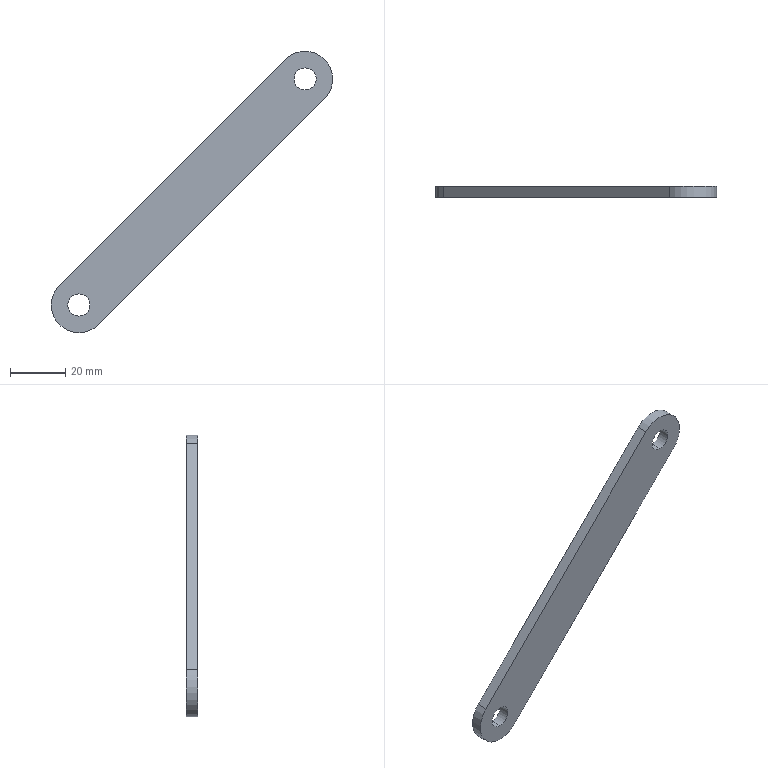Part | SolidWorks | features Extrusion 1 | 1 solid | 11 faces | box 101.635 x 4 x 101.635 mm | volume 10090 mm3 | cylinder 7 | plane 4 | commonest cylinder face diameters 8 x4 20 x3
STEP:
#1=CARTESIAN_POINT('',(-36.47,4.,-44.817));
#2=VERTEX_POINT('',#1);
#3=CARTESIAN_POINT('',(-36.47,4.,-36.817));
#4=VERTEX_POINT('',#3);
#5=CARTESIAN_POINT('',(-36.47,4.,-40.817));
#6=DIRECTION('',(0.,1.,0.));
#7=DIRECTION('',(0.,0.,1.));
#8=AXIS2_PLACEMENT_3D('',#5,#6,#7);
#9=CIRCLE('',#8,4.);
#10=EDGE_CURVE('',#2,#4,#9,.T.);
#11=ORIENTED_EDGE('',*,*,#10,.T.);
#12=CARTESIAN_POINT('',(-36.47,0.,-36.817));
#13=VERTEX_POINT('',#12);
#14=CARTESIAN_POINT('',(-36.47,4.,-36.817));
#15=DIRECTION('',(0.,-1.,0.));
#16=VECTOR('',#15,1000.);
#17=LINE('',#14,#16);
#18=EDGE_CURVE('',#4,#13,#17,.T.);
#19=ORIENTED_EDGE('',*,*,#18,.T.);
#20=CARTESIAN_POINT('',(-36.47,0.,-44.817));
#21=VERTEX_POINT('',#20);
#22=CARTESIAN_POINT('',(-36.47,0.,-40.817));
#23=DIRECTION('',(0.,1.,0.));
#24=DIRECTION('',(0.,0.,1.));
#25=AXIS2_PLACEMENT_3D('',#22,#23,#24);
#26=CIRCLE('',#25,4.);
#27=EDGE_CURVE('',#21,#13,#26,.T.);
#28=ORIENTED_EDGE('',*,*,#27,.F.);
#29=CARTESIAN_POINT('',(-36.47,4.,-44.817));
#30=DIRECTION('',(0.,-1.,0.));
#31=VECTOR('',#30,1000.);
#32=LINE('',#29,#31);
#33=EDGE_CURVE('',#2,#21,#32,.T.);
#34=ORIENTED_EDGE('',*,*,#33,.F.);
#35=EDGE_LOOP('',(#11,#19,#28,#34));
#36=FACE_OUTER_BOUND('',#35,.T.);
#37=CARTESIAN_POINT('',(-36.47,4.,-40.817));
#38=DIRECTION('',(0.,-1.,0.));
#39=DIRECTION('',(0.,0.,-1.));
#40=AXIS2_PLACEMENT_3D('',#37,#38,#39);
#41=CYLINDRICAL_SURFACE('',#40,4.);
#42=ADVANCED_FACE('',(#36),#41,.F.);
#43=CARTESIAN_POINT('',(45.165,4.,36.817));
#44=VERTEX_POINT('',#43);
#45=CARTESIAN_POINT('',(45.165,4.,44.817));
#46=VERTEX_POINT('',#45);
#47=CARTESIAN_POINT('',(45.165,4.,40.817));
#48=DIRECTION('',(0.,1.,0.));
#49=DIRECTION('',(0.,0.,1.));
#50=AXIS2_PLACEMENT_3D('',#47,#48,#49);
#51=CIRCLE('',#50,4.);
#52=EDGE_CURVE('',#44,#46,#51,.T.);
#53=ORIENTED_EDGE('',*,*,#52,.T.);
#54=CARTESIAN_POINT('',(45.165,0.,44.817));
#55=VERTEX_POINT('',#54);
#56=CARTESIAN_POINT('',(45.165,4.,44.817));
#57=DIRECTION('',(0.,-1.,0.));
#58=VECTOR('',#57,1000.);
#59=LINE('',#56,#58);
#60=EDGE_CURVE('',#46,#55,#59,.T.);
#61=ORIENTED_EDGE('',*,*,#60,.T.);
#62=CARTESIAN_POINT('',(45.165,0.,36.817));
#63=VERTEX_POINT('',#62);
#64=CARTESIAN_POINT('',(45.165,0.,40.817));
#65=DIRECTION('',(0.,1.,0.));
#66=DIRECTION('',(0.,0.,1.));
#67=AXIS2_PLACEMENT_3D('',#64,#65,#66);
#68=CIRCLE('',#67,4.);
#69=EDGE_CURVE('',#63,#55,#68,.T.);
#70=ORIENTED_EDGE('',*,*,#69,.F.);
#71=CARTESIAN_POINT('',(45.165,4.,36.817));
#72=DIRECTION('',(0.,-1.,0.));
#73=VECTOR('',#72,1000.);
#74=LINE('',#71,#73);
#75=EDGE_CURVE('',#44,#63,#74,.T.);
#76=ORIENTED_EDGE('',*,*,#75,.F.);
#77=EDGE_LOOP('',(#53,#61,#70,#76));
#78=FACE_OUTER_BOUND('',#77,.T.);
#79=CARTESIAN_POINT('',(45.165,4.,40.817));
#80=DIRECTION('',(0.,-1.,0.));
#81=DIRECTION('',(0.,0.,-1.));
#82=AXIS2_PLACEMENT_3D('',#79,#80,#81);
#83=CYLINDRICAL_SURFACE('',#82,4.);
#84=ADVANCED_FACE('',(#78),#83,.F.);
#85=CARTESIAN_POINT('',(-36.47,4.,-50.817));
#86=VERTEX_POINT('',#85);
#87=CARTESIAN_POINT('',(-43.541,4.,-33.746));
#88=VERTEX_POINT('',#87);
#89=CARTESIAN_POINT('',(-36.47,4.,-40.817));
#90=DIRECTION('',(0.,1.,0.));
#91=DIRECTION('',(0.,0.,1.));
#92=AXIS2_PLACEMENT_3D('',#89,#90,#91);
#93=CIRCLE('',#92,10.);
#94=EDGE_CURVE('',#86,#88,#93,.T.);
#95=ORIENTED_EDGE('',*,*,#94,.F.);
#96=CARTESIAN_POINT('',(-36.47,0.,-50.817));
#97=VERTEX_POINT('',#96);
#98=CARTESIAN_POINT('',(-36.47,4.,-50.817));
#99=DIRECTION('',(0.,-1.,0.));
#100=VECTOR('',#99,1000.);
#101=LINE('',#98,#100);
#102=EDGE_CURVE('',#86,#97,#101,.T.);
#103=ORIENTED_EDGE('',*,*,#102,.T.);
#104=CARTESIAN_POINT('',(-43.541,0.,-33.746));
#105=VERTEX_POINT('',#104);
#106=CARTESIAN_POINT('',(-36.47,0.,-40.817));
#107=DIRECTION('',(0.,1.,0.));
#108=DIRECTION('',(0.,0.,1.));
#109=AXIS2_PLACEMENT_3D('',#106,#107,#108);
#110=CIRCLE('',#109,10.);
#111=EDGE_CURVE('',#97,#105,#110,.T.);
#112=ORIENTED_EDGE('',*,*,#111,.T.);
#113=CARTESIAN_POINT('',(-43.541,4.,-33.746));
#114=DIRECTION('',(0.,-1.,0.));
#115=VECTOR('',#114,1000.);
#116=LINE('',#113,#115);
#117=EDGE_CURVE('',#88,#105,#116,.T.);
#118=ORIENTED_EDGE('',*,*,#117,.F.);
#119=EDGE_LOOP('',(#95,#103,#112,#118));
#120=FACE_OUTER_BOUND('',#119,.T.);
#121=CARTESIAN_POINT('',(-36.47,4.,-40.817));
#122=DIRECTION('',(0.,-1.,0.));
#123=DIRECTION('',(0.,0.,-1.));
#124=AXIS2_PLACEMENT_3D('',#121,#122,#123);
#125=CYLINDRICAL_SURFACE('',#124,10.);
#126=ADVANCED_FACE('',(#120),#125,.T.);
#127=ORIENTED_EDGE('',*,*,#52,.F.);
#128=CARTESIAN_POINT('',(45.165,4.,40.817));
#129=DIRECTION('',(0.,1.,0.));
#130=DIRECTION('',(0.,0.,1.));
#131=AXIS2_PLACEMENT_3D('',#128,#129,#130);
#132=CIRCLE('',#131,4.);
#133=EDGE_CURVE('',#46,#44,#132,.T.);
#134=ORIENTED_EDGE('',*,*,#133,.F.);
#135=EDGE_LOOP('',(#127,#134));
#136=FACE_BOUND('',#135,.T.);
#137=CARTESIAN_POINT('',(38.094,4.,47.889));
#138=VERTEX_POINT('',#137);
#139=CARTESIAN_POINT('',(52.236,4.,33.746));
#140=VERTEX_POINT('',#139);
#141=CARTESIAN_POINT('',(45.165,4.,40.817));
#142=DIRECTION('',(0.,1.,0.));
#143=DIRECTION('',(0.,0.,1.));
#144=AXIS2_PLACEMENT_3D('',#141,#142,#143);
#145=CIRCLE('',#144,10.);
#146=EDGE_CURVE('',#138,#140,#145,.T.);
#147=ORIENTED_EDGE('',*,*,#146,.T.);
#148=CARTESIAN_POINT('',(-29.399,4.,-47.889));
#149=VERTEX_POINT('',#148);
#150=CARTESIAN_POINT('',(52.236,4.,33.746));
#151=DIRECTION('',(-0.7071,0.,-0.7071));
#152=VECTOR('',#151,1000.);
#153=LINE('',#150,#152);
#154=EDGE_CURVE('',#140,#149,#153,.T.);
#155=ORIENTED_EDGE('',*,*,#154,.T.);
#156=CARTESIAN_POINT('',(-36.47,4.,-40.817));
#157=DIRECTION('',(0.,1.,0.));
#158=DIRECTION('',(0.,0.,1.));
#159=AXIS2_PLACEMENT_3D('',#156,#157,#158);
#160=CIRCLE('',#159,10.);
#161=EDGE_CURVE('',#149,#86,#160,.T.);
#162=ORIENTED_EDGE('',*,*,#161,.T.);
#163=ORIENTED_EDGE('',*,*,#94,.T.);
#164=CARTESIAN_POINT('',(38.094,4.,47.889));
#165=DIRECTION('',(0.7071,0.,0.7071));
#166=VECTOR('',#165,1000.);
#167=LINE('',#164,#166);
#168=EDGE_CURVE('',#88,#138,#167,.T.);
#169=ORIENTED_EDGE('',*,*,#168,.T.);
#170=EDGE_LOOP('',(#147,#155,#162,#163,#169));
#171=FACE_OUTER_BOUND('',#170,.T.);
#172=ORIENTED_EDGE('',*,*,#10,.F.);
#173=CARTESIAN_POINT('',(-36.47,4.,-40.817));
#174=DIRECTION('',(0.,1.,0.));
#175=DIRECTION('',(0.,0.,1.));
#176=AXIS2_PLACEMENT_3D('',#173,#174,#175);
#177=CIRCLE('',#176,4.);
#178=EDGE_CURVE('',#4,#2,#177,.T.);
#179=ORIENTED_EDGE('',*,*,#178,.F.);
#180=EDGE_LOOP('',(#172,#179));
#181=FACE_BOUND('',#180,.T.);
#182=CARTESIAN_POINT('',(45.165,4.,40.817));
#183=DIRECTION('',(0.,1.,0.));
#184=DIRECTION('',(0.,0.,1.));
#185=AXIS2_PLACEMENT_3D('',#182,#183,#184);
#186=PLANE('',#185);
#187=ADVANCED_FACE('',(#136,#171,#181),#186,.T.);
#188=CARTESIAN_POINT('',(38.094,0.,47.889));
#189=VERTEX_POINT('',#188);
#190=CARTESIAN_POINT('',(52.236,0.,33.746));
#191=VERTEX_POINT('',#190);
#192=CARTESIAN_POINT('',(45.165,0.,40.817));
#193=DIRECTION('',(0.,1.,0.));
#194=DIRECTION('',(0.,0.,1.));
#195=AXIS2_PLACEMENT_3D('',#192,#193,#194);
#196=CIRCLE('',#195,10.);
#197=EDGE_CURVE('',#189,#191,#196,.T.);
#198=ORIENTED_EDGE('',*,*,#197,.F.);
#199=CARTESIAN_POINT('',(38.094,0.,47.889));
#200=DIRECTION('',(0.7071,0.,0.7071));
#201=VECTOR('',#200,1000.);
#202=LINE('',#199,#201);
#203=EDGE_CURVE('',#105,#189,#202,.T.);
#204=ORIENTED_EDGE('',*,*,#203,.F.);
#205=ORIENTED_EDGE('',*,*,#111,.F.);
#206=CARTESIAN_POINT('',(-29.399,0.,-47.889));
#207=VERTEX_POINT('',#206);
#208=CARTESIAN_POINT('',(-36.47,0.,-40.817));
#209=DIRECTION('',(0.,1.,0.));
#210=DIRECTION('',(0.,0.,1.));
#211=AXIS2_PLACEMENT_3D('',#208,#209,#210);
#212=CIRCLE('',#211,10.);
#213=EDGE_CURVE('',#207,#97,#212,.T.);
#214=ORIENTED_EDGE('',*,*,#213,.F.);
#215=CARTESIAN_POINT('',(52.236,0.,33.746));
#216=DIRECTION('',(-0.7071,0.,-0.7071));
#217=VECTOR('',#216,1000.);
#218=LINE('',#215,#217);
#219=EDGE_CURVE('',#191,#207,#218,.T.);
#220=ORIENTED_EDGE('',*,*,#219,.F.);
#221=EDGE_LOOP('',(#198,#204,#205,#214,#220));
#222=FACE_OUTER_BOUND('',#221,.T.);
#223=ORIENTED_EDGE('',*,*,#69,.T.);
#224=CARTESIAN_POINT('',(45.165,0.,40.817));
#225=DIRECTION('',(0.,1.,0.));
#226=DIRECTION('',(0.,0.,1.));
#227=AXIS2_PLACEMENT_3D('',#224,#225,#226);
#228=CIRCLE('',#227,4.);
#229=EDGE_CURVE('',#55,#63,#228,.T.);
#230=ORIENTED_EDGE('',*,*,#229,.T.);
#231=EDGE_LOOP('',(#223,#230));
#232=FACE_BOUND('',#231,.T.);
#233=ORIENTED_EDGE('',*,*,#27,.T.);
#234=CARTESIAN_POINT('',(-36.47,0.,-40.817));
#235=DIRECTION('',(0.,1.,0.));
#236=DIRECTION('',(0.,0.,1.));
#237=AXIS2_PLACEMENT_3D('',#234,#235,#236);
#238=CIRCLE('',#237,4.);
#239=EDGE_CURVE('',#13,#21,#238,.T.);
#240=ORIENTED_EDGE('',*,*,#239,.T.);
#241=EDGE_LOOP('',(#233,#240));
#242=FACE_BOUND('',#241,.T.);
#243=CARTESIAN_POINT('',(45.165,0.,40.817));
#244=DIRECTION('',(0.,1.,0.));
#245=DIRECTION('',(0.,0.,1.));
#246=AXIS2_PLACEMENT_3D('',#243,#244,#245);
#247=PLANE('',#246);
#248=ADVANCED_FACE('',(#222,#232,#242),#247,.F.);
#249=ORIENTED_EDGE('',*,*,#197,.T.);
#250=CARTESIAN_POINT('',(52.236,4.,33.746));
#251=DIRECTION('',(0.,-1.,0.));
#252=VECTOR('',#251,1000.);
#253=LINE('',#250,#252);
#254=EDGE_CURVE('',#140,#191,#253,.T.);
#255=ORIENTED_EDGE('',*,*,#254,.F.);
#256=ORIENTED_EDGE('',*,*,#146,.F.);
#257=CARTESIAN_POINT('',(38.094,4.,47.889));
#258=DIRECTION('',(0.,-1.,0.));
#259=VECTOR('',#258,1000.);
#260=LINE('',#257,#259);
#261=EDGE_CURVE('',#138,#189,#260,.T.);
#262=ORIENTED_EDGE('',*,*,#261,.T.);
#263=EDGE_LOOP('',(#249,#255,#256,#262));
#264=FACE_OUTER_BOUND('',#263,.T.);
#265=CARTESIAN_POINT('',(45.165,4.,40.817));
#266=DIRECTION('',(0.,-1.,0.));
#267=DIRECTION('',(0.,0.,-1.));
#268=AXIS2_PLACEMENT_3D('',#265,#266,#267);
#269=CYLINDRICAL_SURFACE('',#268,10.);
#270=ADVANCED_FACE('',(#264),#269,.T.);
#271=ORIENTED_EDGE('',*,*,#219,.T.);
#272=CARTESIAN_POINT('',(-29.399,4.,-47.889));
#273=DIRECTION('',(0.,-1.,0.));
#274=VECTOR('',#273,1000.);
#275=LINE('',#272,#274);
#276=EDGE_CURVE('',#149,#207,#275,.T.);
#277=ORIENTED_EDGE('',*,*,#276,.F.);
#278=ORIENTED_EDGE('',*,*,#154,.F.);
#279=ORIENTED_EDGE('',*,*,#254,.T.);
#280=EDGE_LOOP('',(#271,#277,#278,#279));
#281=FACE_OUTER_BOUND('',#280,.T.);
#282=CARTESIAN_POINT('',(52.236,4.,33.746));
#283=DIRECTION('',(-0.7071,0.,0.7071));
#284=DIRECTION('',(0.7071,0.,0.7071));
#285=AXIS2_PLACEMENT_3D('',#282,#283,#284);
#286=PLANE('',#285);
#287=ADVANCED_FACE('',(#281),#286,.F.);
#288=ORIENTED_EDGE('',*,*,#102,.F.);
#289=ORIENTED_EDGE('',*,*,#161,.F.);
#290=ORIENTED_EDGE('',*,*,#276,.T.);
#291=ORIENTED_EDGE('',*,*,#213,.T.);
#292=EDGE_LOOP('',(#288,#289,#290,#291));
#293=FACE_OUTER_BOUND('',#292,.T.);
#294=CARTESIAN_POINT('',(-36.47,4.,-40.817));
#295=DIRECTION('',(0.,-1.,0.));
#296=DIRECTION('',(0.,0.,-1.));
#297=AXIS2_PLACEMENT_3D('',#294,#295,#296);
#298=CYLINDRICAL_SURFACE('',#297,10.);
#299=ADVANCED_FACE('',(#293),#298,.T.);
#300=ORIENTED_EDGE('',*,*,#203,.T.);
#301=ORIENTED_EDGE('',*,*,#261,.F.);
#302=ORIENTED_EDGE('',*,*,#168,.F.);
#303=ORIENTED_EDGE('',*,*,#117,.T.);
#304=EDGE_LOOP('',(#300,#301,#302,#303));
#305=FACE_OUTER_BOUND('',#304,.T.);
#306=CARTESIAN_POINT('',(38.094,4.,47.889));
#307=DIRECTION('',(0.7071,0.,-0.7071));
#308=DIRECTION('',(-0.7071,0.,-0.7071));
#309=AXIS2_PLACEMENT_3D('',#306,#307,#308);
#310=PLANE('',#309);
#311=ADVANCED_FACE('',(#305),#310,.F.);
#312=ORIENTED_EDGE('',*,*,#60,.F.);
#313=ORIENTED_EDGE('',*,*,#133,.T.);
#314=ORIENTED_EDGE('',*,*,#75,.T.);
#315=ORIENTED_EDGE('',*,*,#229,.F.);
#316=EDGE_LOOP('',(#312,#313,#314,#315));
#317=FACE_OUTER_BOUND('',#316,.T.);
#318=CARTESIAN_POINT('',(45.165,4.,40.817));
#319=DIRECTION('',(0.,-1.,0.));
#320=DIRECTION('',(0.,0.,-1.));
#321=AXIS2_PLACEMENT_3D('',#318,#319,#320);
#322=CYLINDRICAL_SURFACE('',#321,4.);
#323=ADVANCED_FACE('',(#317),#322,.F.);
#324=ORIENTED_EDGE('',*,*,#18,.F.);
#325=ORIENTED_EDGE('',*,*,#178,.T.);
#326=ORIENTED_EDGE('',*,*,#33,.T.);
#327=ORIENTED_EDGE('',*,*,#239,.F.);
#328=EDGE_LOOP('',(#324,#325,#326,#327));
#329=FACE_OUTER_BOUND('',#328,.T.);
#330=CARTESIAN_POINT('',(-36.47,4.,-40.817));
#331=DIRECTION('',(0.,-1.,0.));
#332=DIRECTION('',(0.,0.,-1.));
#333=AXIS2_PLACEMENT_3D('',#330,#331,#332);
#334=CYLINDRICAL_SURFACE('',#333,4.);
#335=ADVANCED_FACE('',(#329),#334,.F.);
#336=CLOSED_SHELL('',(#42,#84,#126,#187,#248,#270,#287,#299,#311,#323,#335));
#337=MANIFOLD_SOLID_BREP('',#336);
#338=CARTESIAN_POINT('',(0.,0.,0.));
#339=DIRECTION('',(0.,0.,1.));
#340=DIRECTION('',(1.,0.,0.));
#341=AXIS2_PLACEMENT_3D('',#338,#339,#340);
#342=(LENGTH_UNIT()NAMED_UNIT(*)SI_UNIT(.MILLI.,.METRE.));
#343=UNCERTAINTY_MEASURE_WITH_UNIT(LENGTH_MEASURE(0.00001),#342,'','');
#344=(NAMED_UNIT(*)PLANE_ANGLE_UNIT()SI_UNIT($,.RADIAN.));
#345=(NAMED_UNIT(*)SI_UNIT($,.STERADIAN.)SOLID_ANGLE_UNIT());
#346=(GEOMETRIC_REPRESENTATION_CONTEXT(3)GLOBAL_UNCERTAINTY_ASSIGNED_CONTEXT((#343))GLOBAL_UNIT_ASSIGNED_CONTEXT((#342,#344,#345))REPRESENTATION_CONTEXT('',''));
#347=ADVANCED_BREP_SHAPE_REPRESENTATION('',(#337,#341),#346);